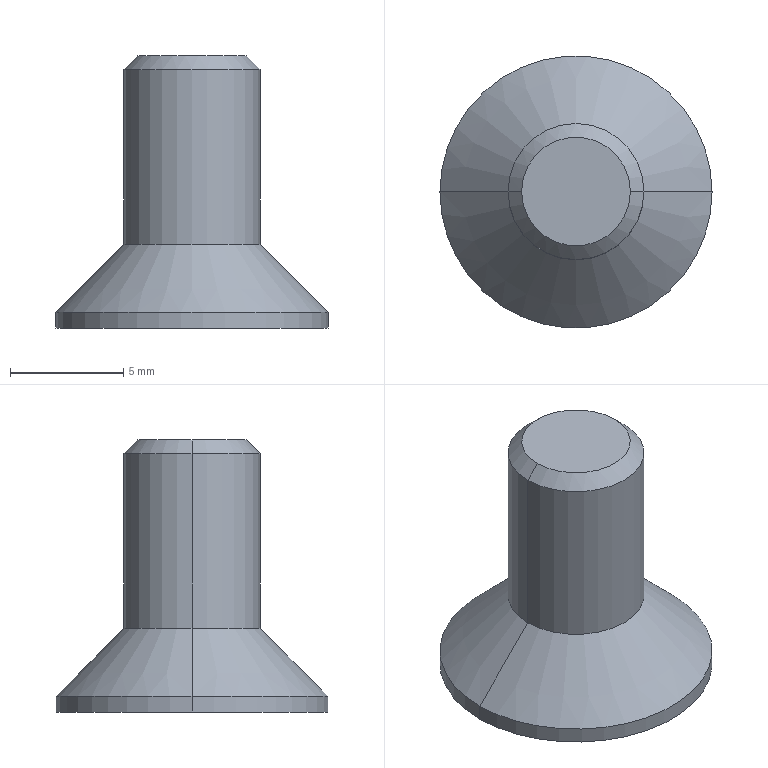Part | STEP file | LE-PJS-M6X12_PN_0009 | 1 solid | 24 faces | box 12 x 12 x 12 mm | volume 458.016 mm3 | plane 14 | cone 6 | cylinder 4 | commonest cylinder face diameters 6 x2 12 x2
STEP:
#1=CARTESIAN_POINT('',(-6.,0.,0.7));
#2=VERTEX_POINT('',#1);
#3=CARTESIAN_POINT('',(6.,0.,0.7));
#4=VERTEX_POINT('',#3);
#5=CARTESIAN_POINT('',(0.,0.,0.7));
#6=DIRECTION('',(0.,0.,-1.));
#7=DIRECTION('',(-1.,0.,0.));
#8=AXIS2_PLACEMENT_3D('',#5,#6,#7);
#9=CIRCLE('',#8,6.);
#10=EDGE_CURVE('',#2,#4,#9,.T.);
#11=ORIENTED_EDGE('',*,*,#10,.T.);
#12=CARTESIAN_POINT('',(6.,0.,0.));
#13=VERTEX_POINT('',#12);
#14=CARTESIAN_POINT('',(6.,0.,3.7));
#15=DIRECTION('',(0.,0.,-1.));
#16=VECTOR('',#15,1000.);
#17=LINE('',#14,#16);
#18=EDGE_CURVE('',#4,#13,#17,.T.);
#19=ORIENTED_EDGE('',*,*,#18,.T.);
#20=CARTESIAN_POINT('',(-6.,0.,0.));
#21=VERTEX_POINT('',#20);
#22=CARTESIAN_POINT('',(0.,0.,0.));
#23=DIRECTION('',(0.,0.,1.));
#24=DIRECTION('',(-1.,0.,0.));
#25=AXIS2_PLACEMENT_3D('',#22,#23,#24);
#26=CIRCLE('',#25,6.);
#27=EDGE_CURVE('',#13,#21,#26,.T.);
#28=ORIENTED_EDGE('',*,*,#27,.T.);
#29=CARTESIAN_POINT('',(-6.,0.,3.7));
#30=DIRECTION('',(0.,0.,-1.));
#31=VECTOR('',#30,1000.);
#32=LINE('',#29,#31);
#33=EDGE_CURVE('',#2,#21,#32,.T.);
#34=ORIENTED_EDGE('',*,*,#33,.F.);
#35=EDGE_LOOP('',(#11,#19,#28,#34));
#36=FACE_OUTER_BOUND('',#35,.T.);
#37=CARTESIAN_POINT('',(0.,0.,3.7));
#38=DIRECTION('',(0.,0.,-1.));
#39=DIRECTION('',(-1.,0.,0.));
#40=AXIS2_PLACEMENT_3D('',#37,#38,#39);
#41=CYLINDRICAL_SURFACE('',#40,6.);
#42=ADVANCED_FACE('',(#36),#41,.T.);
#43=CARTESIAN_POINT('',(-3.,0.,3.7));
#44=VERTEX_POINT('',#43);
#45=CARTESIAN_POINT('',(3.,0.,3.7));
#46=VERTEX_POINT('',#45);
#47=CARTESIAN_POINT('',(0.,0.,3.7));
#48=DIRECTION('',(0.,0.,-1.));
#49=DIRECTION('',(-1.,0.,0.));
#50=AXIS2_PLACEMENT_3D('',#47,#48,#49);
#51=CIRCLE('',#50,3.);
#52=EDGE_CURVE('',#44,#46,#51,.T.);
#53=ORIENTED_EDGE('',*,*,#52,.T.);
#54=CARTESIAN_POINT('',(6.,0.,0.7));
#55=DIRECTION('',(0.7071,0.,-0.7071));
#56=VECTOR('',#55,1000.);
#57=LINE('',#54,#56);
#58=EDGE_CURVE('',#46,#4,#57,.T.);
#59=ORIENTED_EDGE('',*,*,#58,.T.);
#60=ORIENTED_EDGE('',*,*,#10,.F.);
#61=CARTESIAN_POINT('',(-6.,0.,0.7));
#62=DIRECTION('',(-0.7071,0.,-0.7071));
#63=VECTOR('',#62,1000.);
#64=LINE('',#61,#63);
#65=EDGE_CURVE('',#44,#2,#64,.T.);
#66=ORIENTED_EDGE('',*,*,#65,.F.);
#67=EDGE_LOOP('',(#53,#59,#60,#66));
#68=FACE_OUTER_BOUND('',#67,.T.);
#69=CARTESIAN_POINT('',(0.,0.,0.7));
#70=DIRECTION('',(0.,0.,-1.));
#71=DIRECTION('',(-1.,0.,0.));
#72=AXIS2_PLACEMENT_3D('',#69,#70,#71);
#73=CONICAL_SURFACE('',#72,6.,0.7854);
#74=ADVANCED_FACE('',(#68),#73,.T.);
#75=CARTESIAN_POINT('',(-3.,0.,11.4));
#76=VERTEX_POINT('',#75);
#77=CARTESIAN_POINT('',(3.,0.,11.4));
#78=VERTEX_POINT('',#77);
#79=CARTESIAN_POINT('',(0.,0.,11.4));
#80=DIRECTION('',(0.,0.,-1.));
#81=DIRECTION('',(-1.,0.,0.));
#82=AXIS2_PLACEMENT_3D('',#79,#80,#81);
#83=CIRCLE('',#82,3.);
#84=EDGE_CURVE('',#76,#78,#83,.T.);
#85=ORIENTED_EDGE('',*,*,#84,.T.);
#86=CARTESIAN_POINT('',(3.,0.,12.));
#87=DIRECTION('',(0.,0.,-1.));
#88=VECTOR('',#87,1000.);
#89=LINE('',#86,#88);
#90=EDGE_CURVE('',#78,#46,#89,.T.);
#91=ORIENTED_EDGE('',*,*,#90,.T.);
#92=ORIENTED_EDGE('',*,*,#52,.F.);
#93=CARTESIAN_POINT('',(-3.,0.,12.));
#94=DIRECTION('',(0.,0.,-1.));
#95=VECTOR('',#94,1000.);
#96=LINE('',#93,#95);
#97=EDGE_CURVE('',#76,#44,#96,.T.);
#98=ORIENTED_EDGE('',*,*,#97,.F.);
#99=EDGE_LOOP('',(#85,#91,#92,#98));
#100=FACE_OUTER_BOUND('',#99,.T.);
#101=CARTESIAN_POINT('',(0.,0.,12.));
#102=DIRECTION('',(0.,0.,-1.));
#103=DIRECTION('',(-1.,0.,0.));
#104=AXIS2_PLACEMENT_3D('',#101,#102,#103);
#105=CYLINDRICAL_SURFACE('',#104,3.);
#106=ADVANCED_FACE('',(#100),#105,.T.);
#107=CARTESIAN_POINT('',(0.,0.,3.343));
#108=VERTEX_POINT('',#107);
#109=CARTESIAN_POINT('',(-2.5,0.,1.9));
#110=VERTEX_POINT('',#109);
#111=CARTESIAN_POINT('',(-2.5,0.,1.9));
#112=DIRECTION('',(-0.866,0.,-0.5));
#113=VECTOR('',#112,1000.);
#114=LINE('',#111,#113);
#115=EDGE_CURVE('',#108,#110,#114,.T.);
#116=ORIENTED_EDGE('',*,*,#115,.F.);
#117=CARTESIAN_POINT('',(2.5,0.,1.9));
#118=VERTEX_POINT('',#117);
#119=CARTESIAN_POINT('',(2.5,0.,1.9));
#120=DIRECTION('',(0.866,0.,-0.5));
#121=VECTOR('',#120,1000.);
#122=LINE('',#119,#121);
#123=EDGE_CURVE('',#108,#118,#122,.T.);
#124=ORIENTED_EDGE('',*,*,#123,.T.);
#125=CARTESIAN_POINT('',(2.165,-1.25,1.9));
#126=VERTEX_POINT('',#125);
#127=CARTESIAN_POINT('',(0.,0.,1.9));
#128=DIRECTION('',(0.,0.,1.));
#129=DIRECTION('',(-1.,0.,0.));
#130=AXIS2_PLACEMENT_3D('',#127,#128,#129);
#131=CIRCLE('',#130,2.5);
#132=EDGE_CURVE('',#126,#118,#131,.T.);
#133=ORIENTED_EDGE('',*,*,#132,.F.);
#134=CARTESIAN_POINT('',(0.,-2.5,1.9));
#135=VERTEX_POINT('',#134);
#136=CARTESIAN_POINT('',(0.,0.,1.9));
#137=DIRECTION('',(0.,0.,1.));
#138=DIRECTION('',(-1.,0.,0.));
#139=AXIS2_PLACEMENT_3D('',#136,#137,#138);
#140=CIRCLE('',#139,2.5);
#141=EDGE_CURVE('',#135,#126,#140,.T.);
#142=ORIENTED_EDGE('',*,*,#141,.F.);
#143=CARTESIAN_POINT('',(-2.165,-1.25,1.9));
#144=VERTEX_POINT('',#143);
#145=CARTESIAN_POINT('',(0.,0.,1.9));
#146=DIRECTION('',(0.,0.,1.));
#147=DIRECTION('',(-1.,0.,0.));
#148=AXIS2_PLACEMENT_3D('',#145,#146,#147);
#149=CIRCLE('',#148,2.5);
#150=EDGE_CURVE('',#144,#135,#149,.T.);
#151=ORIENTED_EDGE('',*,*,#150,.F.);
#152=CARTESIAN_POINT('',(0.,0.,1.9));
#153=DIRECTION('',(0.,0.,1.));
#154=DIRECTION('',(-1.,0.,0.));
#155=AXIS2_PLACEMENT_3D('',#152,#153,#154);
#156=CIRCLE('',#155,2.5);
#157=EDGE_CURVE('',#110,#144,#156,.T.);
#158=ORIENTED_EDGE('',*,*,#157,.F.);
#159=EDGE_LOOP('',(#116,#124,#133,#142,#151,#158));
#160=FACE_OUTER_BOUND('',#159,.T.);
#161=CARTESIAN_POINT('',(0.,0.,1.9));
#162=DIRECTION('',(0.,0.,-1.));
#163=DIRECTION('',(-1.,0.,0.));
#164=AXIS2_PLACEMENT_3D('',#161,#162,#163);
#165=CONICAL_SURFACE('',#164,2.5,1.047);
#166=ADVANCED_FACE('',(#160),#165,.F.);
#167=CARTESIAN_POINT('',(-2.4,0.,12.));
#168=VERTEX_POINT('',#167);
#169=CARTESIAN_POINT('',(2.4,0.,12.));
#170=VERTEX_POINT('',#169);
#171=CARTESIAN_POINT('',(0.,0.,12.));
#172=DIRECTION('',(0.,0.,-1.));
#173=DIRECTION('',(-1.,0.,0.));
#174=AXIS2_PLACEMENT_3D('',#171,#172,#173);
#175=CIRCLE('',#174,2.4);
#176=EDGE_CURVE('',#168,#170,#175,.T.);
#177=ORIENTED_EDGE('',*,*,#176,.T.);
#178=CARTESIAN_POINT('',(3.,0.,11.4));
#179=DIRECTION('',(0.7071,0.,-0.7071));
#180=VECTOR('',#179,1000.);
#181=LINE('',#178,#180);
#182=EDGE_CURVE('',#170,#78,#181,.T.);
#183=ORIENTED_EDGE('',*,*,#182,.T.);
#184=ORIENTED_EDGE('',*,*,#84,.F.);
#185=CARTESIAN_POINT('',(-3.,0.,11.4));
#186=DIRECTION('',(-0.7071,0.,-0.7071));
#187=VECTOR('',#186,1000.);
#188=LINE('',#185,#187);
#189=EDGE_CURVE('',#168,#76,#188,.T.);
#190=ORIENTED_EDGE('',*,*,#189,.F.);
#191=EDGE_LOOP('',(#177,#183,#184,#190));
#192=FACE_OUTER_BOUND('',#191,.T.);
#193=CARTESIAN_POINT('',(0.,0.,11.4));
#194=DIRECTION('',(0.,0.,-1.));
#195=DIRECTION('',(-1.,0.,0.));
#196=AXIS2_PLACEMENT_3D('',#193,#194,#195);
#197=CONICAL_SURFACE('',#196,3.,0.7854);
#198=ADVANCED_FACE('',(#192),#197,.T.);
#199=CARTESIAN_POINT('',(0.,0.,0.));
#200=DIRECTION('',(0.,0.,1.));
#201=DIRECTION('',(-1.,0.,0.));
#202=AXIS2_PLACEMENT_3D('',#199,#200,#201);
#203=CIRCLE('',#202,6.);
#204=EDGE_CURVE('',#21,#13,#203,.T.);
#205=ORIENTED_EDGE('',*,*,#204,.F.);
#206=ORIENTED_EDGE('',*,*,#27,.F.);
#207=EDGE_LOOP('',(#205,#206));
#208=FACE_OUTER_BOUND('',#207,.T.);
#209=CARTESIAN_POINT('',(-2.887,0.,0.));
#210=VERTEX_POINT('',#209);
#211=CARTESIAN_POINT('',(-1.443,2.5,0.));
#212=VERTEX_POINT('',#211);
#213=CARTESIAN_POINT('',(-2.887,0.,0.));
#214=DIRECTION('',(0.5,0.866,0.));
#215=VECTOR('',#214,1000.);
#216=LINE('',#213,#215);
#217=EDGE_CURVE('',#210,#212,#216,.T.);
#218=ORIENTED_EDGE('',*,*,#217,.F.);
#219=CARTESIAN_POINT('',(-1.443,-2.5,0.));
#220=VERTEX_POINT('',#219);
#221=CARTESIAN_POINT('',(-1.443,-2.5,0.));
#222=DIRECTION('',(-0.5,0.866,0.));
#223=VECTOR('',#222,1000.);
#224=LINE('',#221,#223);
#225=EDGE_CURVE('',#220,#210,#224,.T.);
#226=ORIENTED_EDGE('',*,*,#225,.F.);
#227=CARTESIAN_POINT('',(1.443,-2.5,0.));
#228=VERTEX_POINT('',#227);
#229=CARTESIAN_POINT('',(0.,-2.5,0.));
#230=DIRECTION('',(-1.,0.,0.));
#231=VECTOR('',#230,1000.);
#232=LINE('',#229,#231);
#233=EDGE_CURVE('',#228,#220,#232,.T.);
#234=ORIENTED_EDGE('',*,*,#233,.F.);
#235=CARTESIAN_POINT('',(2.887,0.,0.));
#236=VERTEX_POINT('',#235);
#237=CARTESIAN_POINT('',(2.887,0.,0.));
#238=DIRECTION('',(-0.5,-0.866,0.));
#239=VECTOR('',#238,1000.);
#240=LINE('',#237,#239);
#241=EDGE_CURVE('',#236,#228,#240,.T.);
#242=ORIENTED_EDGE('',*,*,#241,.F.);
#243=CARTESIAN_POINT('',(1.443,2.5,0.));
#244=VERTEX_POINT('',#243);
#245=CARTESIAN_POINT('',(1.443,2.5,0.));
#246=DIRECTION('',(0.5,-0.866,0.));
#247=VECTOR('',#246,1000.);
#248=LINE('',#245,#247);
#249=EDGE_CURVE('',#244,#236,#248,.T.);
#250=ORIENTED_EDGE('',*,*,#249,.F.);
#251=CARTESIAN_POINT('',(0.,2.5,0.));
#252=DIRECTION('',(1.,0.,0.));
#253=VECTOR('',#252,1000.);
#254=LINE('',#251,#253);
#255=EDGE_CURVE('',#212,#244,#254,.T.);
#256=ORIENTED_EDGE('',*,*,#255,.F.);
#257=EDGE_LOOP('',(#218,#226,#234,#242,#250,#256));
#258=FACE_BOUND('',#257,.T.);
#259=CARTESIAN_POINT('',(0.,0.,0.));
#260=DIRECTION('',(0.,0.,1.));
#261=DIRECTION('',(1.,0.,0.));
#262=AXIS2_PLACEMENT_3D('',#259,#260,#261);
#263=PLANE('',#262);
#264=ADVANCED_FACE('',(#208,#258),#263,.F.);
#265=ORIENTED_EDGE('',*,*,#18,.F.);
#266=CARTESIAN_POINT('',(0.,0.,0.7));
#267=DIRECTION('',(0.,0.,-1.));
#268=DIRECTION('',(-1.,0.,0.));
#269=AXIS2_PLACEMENT_3D('',#266,#267,#268);
#270=CIRCLE('',#269,6.);
#271=EDGE_CURVE('',#4,#2,#270,.T.);
#272=ORIENTED_EDGE('',*,*,#271,.T.);
#273=ORIENTED_EDGE('',*,*,#33,.T.);
#274=ORIENTED_EDGE('',*,*,#204,.T.);
#275=EDGE_LOOP('',(#265,#272,#273,#274));
#276=FACE_OUTER_BOUND('',#275,.T.);
#277=CARTESIAN_POINT('',(0.,0.,3.7));
#278=DIRECTION('',(0.,0.,-1.));
#279=DIRECTION('',(-1.,0.,0.));
#280=AXIS2_PLACEMENT_3D('',#277,#278,#279);
#281=CYLINDRICAL_SURFACE('',#280,6.);
#282=ADVANCED_FACE('',(#276),#281,.T.);
#283=CARTESIAN_POINT('',(1.443,2.5,1.9));
#284=VERTEX_POINT('',#283);
#285=CARTESIAN_POINT('',(1.443,2.5,1.9));
#286=DIRECTION('',(0.,0.,-1.));
#287=VECTOR('',#286,1000.);
#288=LINE('',#285,#287);
#289=EDGE_CURVE('',#284,#244,#288,.T.);
#290=ORIENTED_EDGE('',*,*,#289,.F.);
#291=CARTESIAN_POINT('',(0.,2.5,1.9));
#292=VERTEX_POINT('',#291);
#293=CARTESIAN_POINT('',(0.,2.5,1.9));
#294=DIRECTION('',(1.,0.,0.));
#295=VECTOR('',#294,1000.);
#296=LINE('',#293,#295);
#297=EDGE_CURVE('',#292,#284,#296,.T.);
#298=ORIENTED_EDGE('',*,*,#297,.F.);
#299=CARTESIAN_POINT('',(-1.443,2.5,1.9));
#300=VERTEX_POINT('',#299);
#301=CARTESIAN_POINT('',(0.,2.5,1.9));
#302=DIRECTION('',(1.,0.,0.));
#303=VECTOR('',#302,1000.);
#304=LINE('',#301,#303);
#305=EDGE_CURVE('',#300,#292,#304,.T.);
#306=ORIENTED_EDGE('',*,*,#305,.F.);
#307=CARTESIAN_POINT('',(-1.443,2.5,1.9));
#308=DIRECTION('',(0.,0.,1.));
#309=VECTOR('',#308,1000.);
#310=LINE('',#307,#309);
#311=EDGE_CURVE('',#212,#300,#310,.T.);
#312=ORIENTED_EDGE('',*,*,#311,.F.);
#313=ORIENTED_EDGE('',*,*,#255,.T.);
#314=EDGE_LOOP('',(#290,#298,#306,#312,#313));
#315=FACE_OUTER_BOUND('',#314,.T.);
#316=CARTESIAN_POINT('',(-1.443,2.5,1.9));
#317=DIRECTION('',(0.,1.,0.));
#318=DIRECTION('',(0.,0.,1.));
#319=AXIS2_PLACEMENT_3D('',#316,#317,#318);
#320=PLANE('',#319);
#321=ADVANCED_FACE('',(#315),#320,.F.);
#322=ORIENTED_EDGE('',*,*,#311,.T.);
#323=CARTESIAN_POINT('',(-2.165,1.25,1.9));
#324=VERTEX_POINT('',#323);
#325=CARTESIAN_POINT('',(-2.165,1.25,1.9));
#326=DIRECTION('',(0.5,0.866,0.));
#327=VECTOR('',#326,1000.);
#328=LINE('',#325,#327);
#329=EDGE_CURVE('',#324,#300,#328,.T.);
#330=ORIENTED_EDGE('',*,*,#329,.F.);
#331=CARTESIAN_POINT('',(-2.887,0.,1.9));
#332=VERTEX_POINT('',#331);
#333=CARTESIAN_POINT('',(-2.887,0.,1.9));
#334=DIRECTION('',(0.5,0.866,0.));
#335=VECTOR('',#334,1000.);
#336=LINE('',#333,#335);
#337=EDGE_CURVE('',#332,#324,#336,.T.);
#338=ORIENTED_EDGE('',*,*,#337,.F.);
#339=CARTESIAN_POINT('',(-2.887,0.,1.9));
#340=DIRECTION('',(0.,0.,1.));
#341=VECTOR('',#340,1000.);
#342=LINE('',#339,#341);
#343=EDGE_CURVE('',#210,#332,#342,.T.);
#344=ORIENTED_EDGE('',*,*,#343,.F.);
#345=ORIENTED_EDGE('',*,*,#217,.T.);
#346=EDGE_LOOP('',(#322,#330,#338,#344,#345));
#347=FACE_OUTER_BOUND('',#346,.T.);
#348=CARTESIAN_POINT('',(-2.887,0.,1.9));
#349=DIRECTION('',(-0.866,0.5,0.));
#350=DIRECTION('',(-0.5,-0.866,0.));
#351=AXIS2_PLACEMENT_3D('',#348,#349,#350);
#352=PLANE('',#351);
#353=ADVANCED_FACE('',(#347),#352,.F.);
#354=ORIENTED_EDGE('',*,*,#343,.T.);
#355=CARTESIAN_POINT('',(-1.443,-2.5,1.9));
#356=DIRECTION('',(-0.5,0.866,0.));
#357=VECTOR('',#356,1000.);
#358=LINE('',#355,#357);
#359=EDGE_CURVE('',#144,#332,#358,.T.);
#360=ORIENTED_EDGE('',*,*,#359,.F.);
#361=CARTESIAN_POINT('',(-1.443,-2.5,1.9));
#362=VERTEX_POINT('',#361);
#363=CARTESIAN_POINT('',(-1.443,-2.5,1.9));
#364=DIRECTION('',(-0.5,0.866,0.));
#365=VECTOR('',#364,1000.);
#366=LINE('',#363,#365);
#367=EDGE_CURVE('',#362,#144,#366,.T.);
#368=ORIENTED_EDGE('',*,*,#367,.F.);
#369=CARTESIAN_POINT('',(-1.443,-2.5,1.9));
#370=DIRECTION('',(0.,0.,1.));
#371=VECTOR('',#370,1000.);
#372=LINE('',#369,#371);
#373=EDGE_CURVE('',#220,#362,#372,.T.);
#374=ORIENTED_EDGE('',*,*,#373,.F.);
#375=ORIENTED_EDGE('',*,*,#225,.T.);
#376=EDGE_LOOP('',(#354,#360,#368,#374,#375));
#377=FACE_OUTER_BOUND('',#376,.T.);
#378=CARTESIAN_POINT('',(-1.443,-2.5,1.9));
#379=DIRECTION('',(-0.866,-0.5,0.));
#380=DIRECTION('',(0.5,-0.866,0.));
#381=AXIS2_PLACEMENT_3D('',#378,#379,#380);
#382=PLANE('',#381);
#383=ADVANCED_FACE('',(#377),#382,.F.);
#384=ORIENTED_EDGE('',*,*,#373,.T.);
#385=CARTESIAN_POINT('',(0.,-2.5,1.9));
#386=DIRECTION('',(-1.,0.,0.));
#387=VECTOR('',#386,1000.);
#388=LINE('',#385,#387);
#389=EDGE_CURVE('',#135,#362,#388,.T.);
#390=ORIENTED_EDGE('',*,*,#389,.F.);
#391=CARTESIAN_POINT('',(1.443,-2.5,1.9));
#392=VERTEX_POINT('',#391);
#393=CARTESIAN_POINT('',(0.,-2.5,1.9));
#394=DIRECTION('',(-1.,0.,0.));
#395=VECTOR('',#394,1000.);
#396=LINE('',#393,#395);
#397=EDGE_CURVE('',#392,#135,#396,.T.);
#398=ORIENTED_EDGE('',*,*,#397,.F.);
#399=CARTESIAN_POINT('',(1.443,-2.5,1.9));
#400=DIRECTION('',(0.,0.,1.));
#401=VECTOR('',#400,1000.);
#402=LINE('',#399,#401);
#403=EDGE_CURVE('',#228,#392,#402,.T.);
#404=ORIENTED_EDGE('',*,*,#403,.F.);
#405=ORIENTED_EDGE('',*,*,#233,.T.);
#406=EDGE_LOOP('',(#384,#390,#398,#404,#405));
#407=FACE_OUTER_BOUND('',#406,.T.);
#408=CARTESIAN_POINT('',(1.443,-2.5,1.9));
#409=DIRECTION('',(0.,-1.,0.));
#410=DIRECTION('',(1.,0.,0.));
#411=AXIS2_PLACEMENT_3D('',#408,#409,#410);
#412=PLANE('',#411);
#413=ADVANCED_FACE('',(#407),#412,.F.);
#414=ORIENTED_EDGE('',*,*,#403,.T.);
#415=CARTESIAN_POINT('',(2.165,-1.25,1.9));
#416=DIRECTION('',(-0.5,-0.866,0.));
#417=VECTOR('',#416,1000.);
#418=LINE('',#415,#417);
#419=EDGE_CURVE('',#126,#392,#418,.T.);
#420=ORIENTED_EDGE('',*,*,#419,.F.);
#421=CARTESIAN_POINT('',(2.887,0.,1.9));
#422=VERTEX_POINT('',#421);
#423=CARTESIAN_POINT('',(2.887,0.,1.9));
#424=DIRECTION('',(-0.5,-0.866,0.));
#425=VECTOR('',#424,1000.);
#426=LINE('',#423,#425);
#427=EDGE_CURVE('',#422,#126,#426,.T.);
#428=ORIENTED_EDGE('',*,*,#427,.F.);
#429=CARTESIAN_POINT('',(2.887,0.,1.9));
#430=DIRECTION('',(0.,0.,1.));
#431=VECTOR('',#430,1000.);
#432=LINE('',#429,#431);
#433=EDGE_CURVE('',#236,#422,#432,.T.);
#434=ORIENTED_EDGE('',*,*,#433,.F.);
#435=ORIENTED_EDGE('',*,*,#241,.T.);
#436=EDGE_LOOP('',(#414,#420,#428,#434,#435));
#437=FACE_OUTER_BOUND('',#436,.T.);
#438=CARTESIAN_POINT('',(2.887,0.,1.9));
#439=DIRECTION('',(0.866,-0.5,0.));
#440=DIRECTION('',(0.5,0.866,0.));
#441=AXIS2_PLACEMENT_3D('',#438,#439,#440);
#442=PLANE('',#441);
#443=ADVANCED_FACE('',(#437),#442,.F.);
#444=ORIENTED_EDGE('',*,*,#433,.T.);
#445=CARTESIAN_POINT('',(2.165,1.25,1.9));
#446=VERTEX_POINT('',#445);
#447=CARTESIAN_POINT('',(1.443,2.5,1.9));
#448=DIRECTION('',(0.5,-0.866,0.));
#449=VECTOR('',#448,1000.);
#450=LINE('',#447,#449);
#451=EDGE_CURVE('',#446,#422,#450,.T.);
#452=ORIENTED_EDGE('',*,*,#451,.F.);
#453=CARTESIAN_POINT('',(1.443,2.5,1.9));
#454=DIRECTION('',(0.5,-0.866,0.));
#455=VECTOR('',#454,1000.);
#456=LINE('',#453,#455);
#457=EDGE_CURVE('',#284,#446,#456,.T.);
#458=ORIENTED_EDGE('',*,*,#457,.F.);
#459=ORIENTED_EDGE('',*,*,#289,.T.);
#460=ORIENTED_EDGE('',*,*,#249,.T.);
#461=EDGE_LOOP('',(#444,#452,#458,#459,#460));
#462=FACE_OUTER_BOUND('',#461,.T.);
#463=CARTESIAN_POINT('',(1.443,2.5,1.9));
#464=DIRECTION('',(0.866,0.5,0.));
#465=DIRECTION('',(-0.5,0.866,0.));
#466=AXIS2_PLACEMENT_3D('',#463,#464,#465);
#467=PLANE('',#466);
#468=ADVANCED_FACE('',(#462),#467,.F.);
#469=ORIENTED_EDGE('',*,*,#58,.F.);
#470=CARTESIAN_POINT('',(0.,0.,3.7));
#471=DIRECTION('',(0.,0.,-1.));
#472=DIRECTION('',(-1.,0.,0.));
#473=AXIS2_PLACEMENT_3D('',#470,#471,#472);
#474=CIRCLE('',#473,3.);
#475=EDGE_CURVE('',#46,#44,#474,.T.);
#476=ORIENTED_EDGE('',*,*,#475,.T.);
#477=ORIENTED_EDGE('',*,*,#65,.T.);
#478=ORIENTED_EDGE('',*,*,#271,.F.);
#479=EDGE_LOOP('',(#469,#476,#477,#478));
#480=FACE_OUTER_BOUND('',#479,.T.);
#481=CARTESIAN_POINT('',(0.,0.,0.7));
#482=DIRECTION('',(0.,0.,-1.));
#483=DIRECTION('',(-1.,0.,0.));
#484=AXIS2_PLACEMENT_3D('',#481,#482,#483);
#485=CONICAL_SURFACE('',#484,6.,0.7854);
#486=ADVANCED_FACE('',(#480),#485,.T.);
#487=ORIENTED_EDGE('',*,*,#337,.T.);
#488=CARTESIAN_POINT('',(0.,0.,1.9));
#489=DIRECTION('',(0.,0.,1.));
#490=DIRECTION('',(-1.,0.,0.));
#491=AXIS2_PLACEMENT_3D('',#488,#489,#490);
#492=CIRCLE('',#491,2.5);
#493=EDGE_CURVE('',#324,#110,#492,.T.);
#494=ORIENTED_EDGE('',*,*,#493,.T.);
#495=ORIENTED_EDGE('',*,*,#157,.T.);
#496=ORIENTED_EDGE('',*,*,#359,.T.);
#497=EDGE_LOOP('',(#487,#494,#495,#496));
#498=FACE_OUTER_BOUND('',#497,.T.);
#499=CARTESIAN_POINT('',(0.,0.,1.9));
#500=DIRECTION('',(0.,0.,-1.));
#501=DIRECTION('',(-1.,0.,0.));
#502=AXIS2_PLACEMENT_3D('',#499,#500,#501);
#503=PLANE('',#502);
#504=ADVANCED_FACE('',(#498),#503,.T.);
#505=ORIENTED_EDGE('',*,*,#427,.T.);
#506=ORIENTED_EDGE('',*,*,#132,.T.);
#507=CARTESIAN_POINT('',(0.,0.,1.9));
#508=DIRECTION('',(0.,0.,1.));
#509=DIRECTION('',(-1.,0.,0.));
#510=AXIS2_PLACEMENT_3D('',#507,#508,#509);
#511=CIRCLE('',#510,2.5);
#512=EDGE_CURVE('',#118,#446,#511,.T.);
#513=ORIENTED_EDGE('',*,*,#512,.T.);
#514=ORIENTED_EDGE('',*,*,#451,.T.);
#515=EDGE_LOOP('',(#505,#506,#513,#514));
#516=FACE_OUTER_BOUND('',#515,.T.);
#517=CARTESIAN_POINT('',(0.,0.,1.9));
#518=DIRECTION('',(0.,0.,-1.));
#519=DIRECTION('',(-1.,0.,0.));
#520=AXIS2_PLACEMENT_3D('',#517,#518,#519);
#521=PLANE('',#520);
#522=ADVANCED_FACE('',(#516),#521,.T.);
#523=ORIENTED_EDGE('',*,*,#297,.T.);
#524=ORIENTED_EDGE('',*,*,#457,.T.);
#525=CARTESIAN_POINT('',(0.,0.,1.9));
#526=DIRECTION('',(0.,0.,1.));
#527=DIRECTION('',(-1.,0.,0.));
#528=AXIS2_PLACEMENT_3D('',#525,#526,#527);
#529=CIRCLE('',#528,2.5);
#530=EDGE_CURVE('',#446,#292,#529,.T.);
#531=ORIENTED_EDGE('',*,*,#530,.T.);
#532=EDGE_LOOP('',(#523,#524,#531));
#533=FACE_OUTER_BOUND('',#532,.T.);
#534=CARTESIAN_POINT('',(0.,0.,1.9));
#535=DIRECTION('',(0.,0.,-1.));
#536=DIRECTION('',(-1.,0.,0.));
#537=AXIS2_PLACEMENT_3D('',#534,#535,#536);
#538=PLANE('',#537);
#539=ADVANCED_FACE('',(#533),#538,.T.);
#540=ORIENTED_EDGE('',*,*,#90,.F.);
#541=CARTESIAN_POINT('',(0.,0.,11.4));
#542=DIRECTION('',(0.,0.,-1.));
#543=DIRECTION('',(-1.,0.,0.));
#544=AXIS2_PLACEMENT_3D('',#541,#542,#543);
#545=CIRCLE('',#544,3.);
#546=EDGE_CURVE('',#78,#76,#545,.T.);
#547=ORIENTED_EDGE('',*,*,#546,.T.);
#548=ORIENTED_EDGE('',*,*,#97,.T.);
#549=ORIENTED_EDGE('',*,*,#475,.F.);
#550=EDGE_LOOP('',(#540,#547,#548,#549));
#551=FACE_OUTER_BOUND('',#550,.T.);
#552=CARTESIAN_POINT('',(0.,0.,12.));
#553=DIRECTION('',(0.,0.,-1.));
#554=DIRECTION('',(-1.,0.,0.));
#555=AXIS2_PLACEMENT_3D('',#552,#553,#554);
#556=CYLINDRICAL_SURFACE('',#555,3.);
#557=ADVANCED_FACE('',(#551),#556,.T.);
#558=ORIENTED_EDGE('',*,*,#123,.F.);
#559=ORIENTED_EDGE('',*,*,#115,.T.);
#560=ORIENTED_EDGE('',*,*,#493,.F.);
#561=CARTESIAN_POINT('',(0.,0.,1.9));
#562=DIRECTION('',(0.,0.,1.));
#563=DIRECTION('',(-1.,0.,0.));
#564=AXIS2_PLACEMENT_3D('',#561,#562,#563);
#565=CIRCLE('',#564,2.5);
#566=EDGE_CURVE('',#292,#324,#565,.T.);
#567=ORIENTED_EDGE('',*,*,#566,.F.);
#568=ORIENTED_EDGE('',*,*,#530,.F.);
#569=ORIENTED_EDGE('',*,*,#512,.F.);
#570=EDGE_LOOP('',(#558,#559,#560,#567,#568,#569));
#571=FACE_OUTER_BOUND('',#570,.T.);
#572=CARTESIAN_POINT('',(0.,0.,1.9));
#573=DIRECTION('',(0.,0.,-1.));
#574=DIRECTION('',(-1.,0.,0.));
#575=AXIS2_PLACEMENT_3D('',#572,#573,#574);
#576=CONICAL_SURFACE('',#575,2.5,1.047);
#577=ADVANCED_FACE('',(#571),#576,.F.);
#578=ORIENTED_EDGE('',*,*,#182,.F.);
#579=CARTESIAN_POINT('',(0.,0.,12.));
#580=DIRECTION('',(0.,0.,-1.));
#581=DIRECTION('',(-1.,0.,0.));
#582=AXIS2_PLACEMENT_3D('',#579,#580,#581);
#583=CIRCLE('',#582,2.4);
#584=EDGE_CURVE('',#170,#168,#583,.T.);
#585=ORIENTED_EDGE('',*,*,#584,.T.);
#586=ORIENTED_EDGE('',*,*,#189,.T.);
#587=ORIENTED_EDGE('',*,*,#546,.F.);
#588=EDGE_LOOP('',(#578,#585,#586,#587));
#589=FACE_OUTER_BOUND('',#588,.T.);
#590=CARTESIAN_POINT('',(0.,0.,11.4));
#591=DIRECTION('',(0.,0.,-1.));
#592=DIRECTION('',(-1.,0.,0.));
#593=AXIS2_PLACEMENT_3D('',#590,#591,#592);
#594=CONICAL_SURFACE('',#593,3.,0.7854);
#595=ADVANCED_FACE('',(#589),#594,.T.);
#596=ORIENTED_EDGE('',*,*,#329,.T.);
#597=ORIENTED_EDGE('',*,*,#305,.T.);
#598=ORIENTED_EDGE('',*,*,#566,.T.);
#599=EDGE_LOOP('',(#596,#597,#598));
#600=FACE_OUTER_BOUND('',#599,.T.);
#601=CARTESIAN_POINT('',(0.,0.,1.9));
#602=DIRECTION('',(0.,0.,-1.));
#603=DIRECTION('',(-1.,0.,0.));
#604=AXIS2_PLACEMENT_3D('',#601,#602,#603);
#605=PLANE('',#604);
#606=ADVANCED_FACE('',(#600),#605,.T.);
#607=ORIENTED_EDGE('',*,*,#176,.F.);
#608=ORIENTED_EDGE('',*,*,#584,.F.);
#609=EDGE_LOOP('',(#607,#608));
#610=FACE_OUTER_BOUND('',#609,.T.);
#611=CARTESIAN_POINT('',(0.,0.,12.));
#612=DIRECTION('',(0.,0.,1.));
#613=DIRECTION('',(1.,0.,0.));
#614=AXIS2_PLACEMENT_3D('',#611,#612,#613);
#615=PLANE('',#614);
#616=ADVANCED_FACE('',(#610),#615,.T.);
#617=ORIENTED_EDGE('',*,*,#419,.T.);
#618=ORIENTED_EDGE('',*,*,#397,.T.);
#619=ORIENTED_EDGE('',*,*,#141,.T.);
#620=EDGE_LOOP('',(#617,#618,#619));
#621=FACE_OUTER_BOUND('',#620,.T.);
#622=CARTESIAN_POINT('',(0.,0.,1.9));
#623=DIRECTION('',(0.,0.,-1.));
#624=DIRECTION('',(-1.,0.,0.));
#625=AXIS2_PLACEMENT_3D('',#622,#623,#624);
#626=PLANE('',#625);
#627=ADVANCED_FACE('',(#621),#626,.T.);
#628=ORIENTED_EDGE('',*,*,#389,.T.);
#629=ORIENTED_EDGE('',*,*,#367,.T.);
#630=ORIENTED_EDGE('',*,*,#150,.T.);
#631=EDGE_LOOP('',(#628,#629,#630));
#632=FACE_OUTER_BOUND('',#631,.T.);
#633=CARTESIAN_POINT('',(0.,0.,1.9));
#634=DIRECTION('',(0.,0.,-1.));
#635=DIRECTION('',(-1.,0.,0.));
#636=AXIS2_PLACEMENT_3D('',#633,#634,#635);
#637=PLANE('',#636);
#638=ADVANCED_FACE('',(#632),#637,.T.);
#639=CLOSED_SHELL('',(#42,#74,#106,#166,#198,#264,#282,#321,#353,#383,#413,#443,#468,#486,#504,#522,#539,#557,#577,#595,#606,#616,#627,#638));
#640=MANIFOLD_SOLID_BREP('',#639);
#641=CARTESIAN_POINT('',(0.,0.,0.));
#642=DIRECTION('',(0.,0.,1.));
#643=DIRECTION('',(1.,0.,0.));
#644=AXIS2_PLACEMENT_3D('',#641,#642,#643);
#645=(LENGTH_UNIT()NAMED_UNIT(*)SI_UNIT(.MILLI.,.METRE.));
#646=UNCERTAINTY_MEASURE_WITH_UNIT(LENGTH_MEASURE(0.00001),#645,'','');
#647=(NAMED_UNIT(*)PLANE_ANGLE_UNIT()SI_UNIT($,.RADIAN.));
#648=(NAMED_UNIT(*)SI_UNIT($,.STERADIAN.)SOLID_ANGLE_UNIT());
#649=(GEOMETRIC_REPRESENTATION_CONTEXT(3)GLOBAL_UNCERTAINTY_ASSIGNED_CONTEXT((#646))GLOBAL_UNIT_ASSIGNED_CONTEXT((#645,#647,#648))REPRESENTATION_CONTEXT('',''));
#650=ADVANCED_BREP_SHAPE_REPRESENTATION('',(#640,#644),#649);